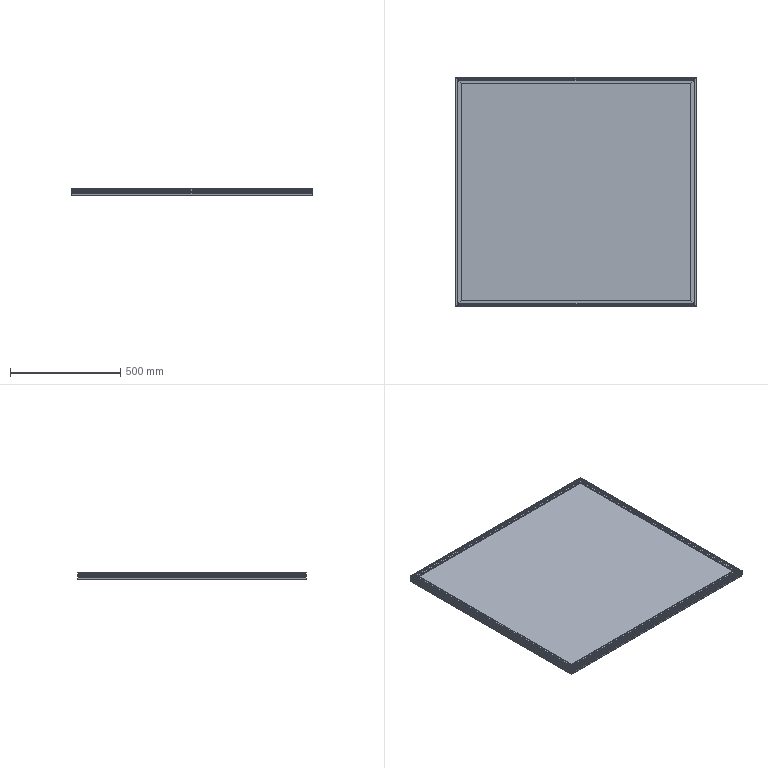Part | SolidWorks | features ICE 1, WeldMemberFeat 1, WeldmentFeature 1 | 5 solids | 272 faces | box 1095 x 1035 x 30 mm | volume 24245961 mm3 | plane 222 | cylinder 50 | commonest cylinder face diameters 0.4 x26 2 x16 1 x8